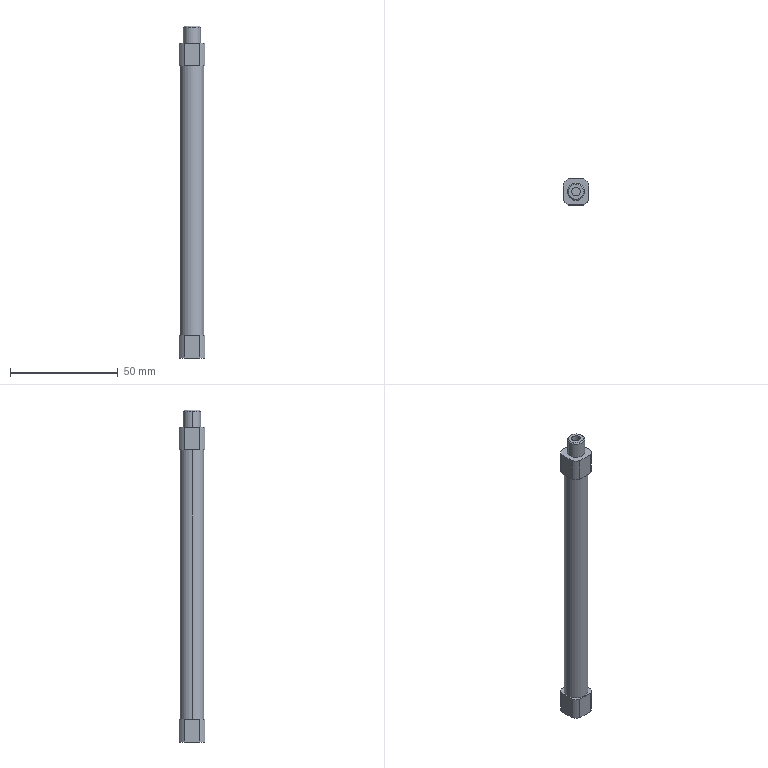Part | Creo | features CURVE 3, DATUM PLANE 3, PROTRUSION 2, CHAMFER 1, COORDINATE SYSTEM 1, CUT 1 | 1 solid | 30 faces | volume 15001 mm3 | plane 14 | cylinder 14 | cone 2 | commonest cylinder face diameters 14 x8 4 x2 8 x2 11 x2